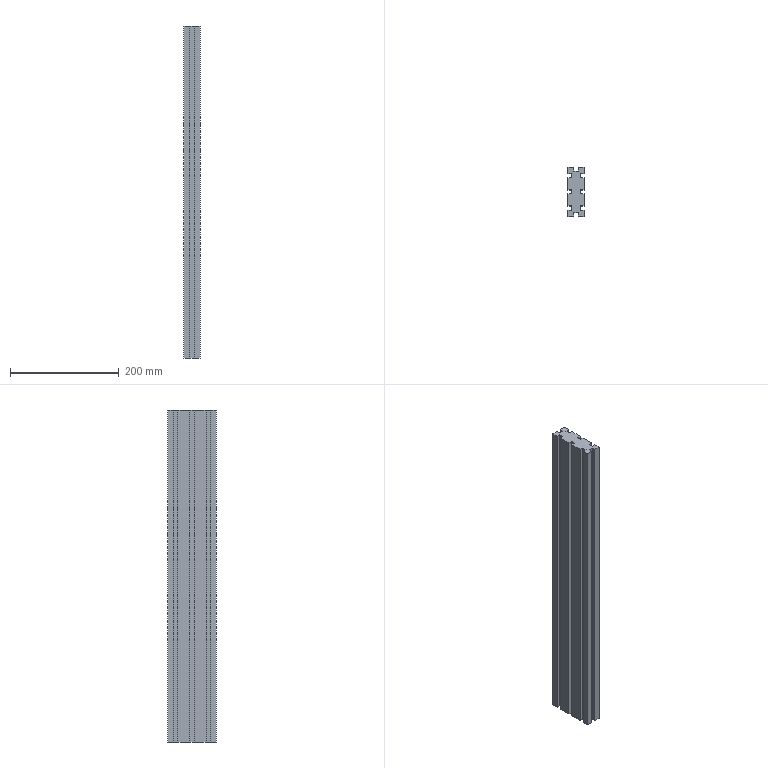Part | SolidWorks | features BaseBody 1 | 1 solid | 38 faces | box 30 x 90 x 610 mm | volume 1373720 mm3 | plane 38
STEP:
#1=CARTESIAN_POINT('',(8.,-4.,610.));
#2=VERTEX_POINT('',#1);
#3=CARTESIAN_POINT('',(15.,-4.,610.));
#4=VERTEX_POINT('',#3);
#5=CARTESIAN_POINT('',(8.,-4.,610.));
#6=DIRECTION('',(1.,0.,0.));
#7=VECTOR('',#6,1000.);
#8=LINE('',#5,#7);
#9=EDGE_CURVE('',#2,#4,#8,.T.);
#10=ORIENTED_EDGE('',*,*,#9,.T.);
#11=CARTESIAN_POINT('',(15.,-4.,0.));
#12=VERTEX_POINT('',#11);
#13=CARTESIAN_POINT('',(15.,-4.,0.));
#14=DIRECTION('',(0.,0.,1.));
#15=VECTOR('',#14,1000.);
#16=LINE('',#13,#15);
#17=EDGE_CURVE('',#12,#4,#16,.T.);
#18=ORIENTED_EDGE('',*,*,#17,.F.);
#19=CARTESIAN_POINT('',(8.,-4.,0.));
#20=VERTEX_POINT('',#19);
#21=CARTESIAN_POINT('',(8.,-4.,0.));
#22=DIRECTION('',(1.,0.,0.));
#23=VECTOR('',#22,1000.);
#24=LINE('',#21,#23);
#25=EDGE_CURVE('',#20,#12,#24,.T.);
#26=ORIENTED_EDGE('',*,*,#25,.F.);
#27=CARTESIAN_POINT('',(8.,-4.,0.));
#28=DIRECTION('',(0.,0.,1.));
#29=VECTOR('',#28,1000.);
#30=LINE('',#27,#29);
#31=EDGE_CURVE('',#20,#2,#30,.T.);
#32=ORIENTED_EDGE('',*,*,#31,.T.);
#33=EDGE_LOOP('',(#10,#18,#26,#32));
#34=FACE_OUTER_BOUND('',#33,.T.);
#35=CARTESIAN_POINT('',(8.,-4.,0.));
#36=DIRECTION('',(0.,-1.,0.));
#37=DIRECTION('',(0.,0.,-1.));
#38=AXIS2_PLACEMENT_3D('',#35,#36,#37);
#39=PLANE('',#38);
#40=ADVANCED_FACE('',(#34),#39,.F.);
#41=CARTESIAN_POINT('',(15.,4.,610.));
#42=VERTEX_POINT('',#41);
#43=CARTESIAN_POINT('',(8.,4.,610.));
#44=VERTEX_POINT('',#43);
#45=CARTESIAN_POINT('',(8.,4.,610.));
#46=DIRECTION('',(-1.,0.,0.));
#47=VECTOR('',#46,1000.);
#48=LINE('',#45,#47);
#49=EDGE_CURVE('',#42,#44,#48,.T.);
#50=ORIENTED_EDGE('',*,*,#49,.T.);
#51=CARTESIAN_POINT('',(8.,4.,0.));
#52=VERTEX_POINT('',#51);
#53=CARTESIAN_POINT('',(8.,4.,0.));
#54=DIRECTION('',(0.,0.,1.));
#55=VECTOR('',#54,1000.);
#56=LINE('',#53,#55);
#57=EDGE_CURVE('',#52,#44,#56,.T.);
#58=ORIENTED_EDGE('',*,*,#57,.F.);
#59=CARTESIAN_POINT('',(15.,4.,0.));
#60=VERTEX_POINT('',#59);
#61=CARTESIAN_POINT('',(8.,4.,0.));
#62=DIRECTION('',(-1.,0.,0.));
#63=VECTOR('',#62,1000.);
#64=LINE('',#61,#63);
#65=EDGE_CURVE('',#60,#52,#64,.T.);
#66=ORIENTED_EDGE('',*,*,#65,.F.);
#67=CARTESIAN_POINT('',(15.,4.,0.));
#68=DIRECTION('',(0.,0.,1.));
#69=VECTOR('',#68,1000.);
#70=LINE('',#67,#69);
#71=EDGE_CURVE('',#60,#42,#70,.T.);
#72=ORIENTED_EDGE('',*,*,#71,.T.);
#73=EDGE_LOOP('',(#50,#58,#66,#72));
#74=FACE_OUTER_BOUND('',#73,.T.);
#75=CARTESIAN_POINT('',(8.,4.,0.));
#76=DIRECTION('',(0.,1.,0.));
#77=DIRECTION('',(1.,0.,0.));
#78=AXIS2_PLACEMENT_3D('',#75,#76,#77);
#79=PLANE('',#78);
#80=ADVANCED_FACE('',(#74),#79,.F.);
#81=CARTESIAN_POINT('',(8.,-4.,610.));
#82=DIRECTION('',(0.,-1.,0.));
#83=VECTOR('',#82,1000.);
#84=LINE('',#81,#83);
#85=EDGE_CURVE('',#44,#2,#84,.T.);
#86=ORIENTED_EDGE('',*,*,#85,.T.);
#87=ORIENTED_EDGE('',*,*,#31,.F.);
#88=CARTESIAN_POINT('',(8.,-4.,0.));
#89=DIRECTION('',(0.,-1.,0.));
#90=VECTOR('',#89,1000.);
#91=LINE('',#88,#90);
#92=EDGE_CURVE('',#52,#20,#91,.T.);
#93=ORIENTED_EDGE('',*,*,#92,.F.);
#94=ORIENTED_EDGE('',*,*,#57,.T.);
#95=EDGE_LOOP('',(#86,#87,#93,#94));
#96=FACE_OUTER_BOUND('',#95,.T.);
#97=CARTESIAN_POINT('',(8.,-4.,0.));
#98=DIRECTION('',(-1.,0.,0.));
#99=DIRECTION('',(0.,0.,1.));
#100=AXIS2_PLACEMENT_3D('',#97,#98,#99);
#101=PLANE('',#100);
#102=ADVANCED_FACE('',(#96),#101,.F.);
#103=CARTESIAN_POINT('',(-15.,-4.,610.));
#104=VERTEX_POINT('',#103);
#105=CARTESIAN_POINT('',(-8.,-4.,610.));
#106=VERTEX_POINT('',#105);
#107=CARTESIAN_POINT('',(-15.,-4.,610.));
#108=DIRECTION('',(1.,0.,0.));
#109=VECTOR('',#108,1000.);
#110=LINE('',#107,#109);
#111=EDGE_CURVE('',#104,#106,#110,.T.);
#112=ORIENTED_EDGE('',*,*,#111,.T.);
#113=CARTESIAN_POINT('',(-8.,-4.,0.));
#114=VERTEX_POINT('',#113);
#115=CARTESIAN_POINT('',(-8.,-4.,0.));
#116=DIRECTION('',(0.,0.,1.));
#117=VECTOR('',#116,1000.);
#118=LINE('',#115,#117);
#119=EDGE_CURVE('',#114,#106,#118,.T.);
#120=ORIENTED_EDGE('',*,*,#119,.F.);
#121=CARTESIAN_POINT('',(-15.,-4.,0.));
#122=VERTEX_POINT('',#121);
#123=CARTESIAN_POINT('',(-15.,-4.,0.));
#124=DIRECTION('',(1.,0.,0.));
#125=VECTOR('',#124,1000.);
#126=LINE('',#123,#125);
#127=EDGE_CURVE('',#122,#114,#126,.T.);
#128=ORIENTED_EDGE('',*,*,#127,.F.);
#129=CARTESIAN_POINT('',(-15.,-4.,0.));
#130=DIRECTION('',(0.,0.,1.));
#131=VECTOR('',#130,1000.);
#132=LINE('',#129,#131);
#133=EDGE_CURVE('',#122,#104,#132,.T.);
#134=ORIENTED_EDGE('',*,*,#133,.T.);
#135=EDGE_LOOP('',(#112,#120,#128,#134));
#136=FACE_OUTER_BOUND('',#135,.T.);
#137=CARTESIAN_POINT('',(-15.,-4.,0.));
#138=DIRECTION('',(0.,-1.,0.));
#139=DIRECTION('',(0.,0.,-1.));
#140=AXIS2_PLACEMENT_3D('',#137,#138,#139);
#141=PLANE('',#140);
#142=ADVANCED_FACE('',(#136),#141,.F.);
#143=CARTESIAN_POINT('',(-8.,4.,610.));
#144=VERTEX_POINT('',#143);
#145=CARTESIAN_POINT('',(-8.,-4.,610.));
#146=DIRECTION('',(0.,1.,0.));
#147=VECTOR('',#146,1000.);
#148=LINE('',#145,#147);
#149=EDGE_CURVE('',#106,#144,#148,.T.);
#150=ORIENTED_EDGE('',*,*,#149,.T.);
#151=CARTESIAN_POINT('',(-8.,4.,0.));
#152=VERTEX_POINT('',#151);
#153=CARTESIAN_POINT('',(-8.,4.,0.));
#154=DIRECTION('',(0.,0.,1.));
#155=VECTOR('',#154,1000.);
#156=LINE('',#153,#155);
#157=EDGE_CURVE('',#152,#144,#156,.T.);
#158=ORIENTED_EDGE('',*,*,#157,.F.);
#159=CARTESIAN_POINT('',(-8.,-4.,0.));
#160=DIRECTION('',(0.,1.,0.));
#161=VECTOR('',#160,1000.);
#162=LINE('',#159,#161);
#163=EDGE_CURVE('',#114,#152,#162,.T.);
#164=ORIENTED_EDGE('',*,*,#163,.F.);
#165=ORIENTED_EDGE('',*,*,#119,.T.);
#166=EDGE_LOOP('',(#150,#158,#164,#165));
#167=FACE_OUTER_BOUND('',#166,.T.);
#168=CARTESIAN_POINT('',(-8.,-4.,0.));
#169=DIRECTION('',(1.,0.,0.));
#170=DIRECTION('',(0.,1.,0.));
#171=AXIS2_PLACEMENT_3D('',#168,#169,#170);
#172=PLANE('',#171);
#173=ADVANCED_FACE('',(#167),#172,.F.);
#174=CARTESIAN_POINT('',(-15.,4.,610.));
#175=VERTEX_POINT('',#174);
#176=CARTESIAN_POINT('',(-15.,4.,610.));
#177=DIRECTION('',(-1.,0.,0.));
#178=VECTOR('',#177,1000.);
#179=LINE('',#176,#178);
#180=EDGE_CURVE('',#144,#175,#179,.T.);
#181=ORIENTED_EDGE('',*,*,#180,.T.);
#182=CARTESIAN_POINT('',(-15.,4.,0.));
#183=VERTEX_POINT('',#182);
#184=CARTESIAN_POINT('',(-15.,4.,0.));
#185=DIRECTION('',(0.,0.,1.));
#186=VECTOR('',#185,1000.);
#187=LINE('',#184,#186);
#188=EDGE_CURVE('',#183,#175,#187,.T.);
#189=ORIENTED_EDGE('',*,*,#188,.F.);
#190=CARTESIAN_POINT('',(-15.,4.,0.));
#191=DIRECTION('',(-1.,0.,0.));
#192=VECTOR('',#191,1000.);
#193=LINE('',#190,#192);
#194=EDGE_CURVE('',#152,#183,#193,.T.);
#195=ORIENTED_EDGE('',*,*,#194,.F.);
#196=ORIENTED_EDGE('',*,*,#157,.T.);
#197=EDGE_LOOP('',(#181,#189,#195,#196));
#198=FACE_OUTER_BOUND('',#197,.T.);
#199=CARTESIAN_POINT('',(-15.,4.,0.));
#200=DIRECTION('',(0.,1.,0.));
#201=DIRECTION('',(1.,0.,0.));
#202=AXIS2_PLACEMENT_3D('',#199,#200,#201);
#203=PLANE('',#202);
#204=ADVANCED_FACE('',(#198),#203,.F.);
#205=CARTESIAN_POINT('',(15.,-26.,610.));
#206=VERTEX_POINT('',#205);
#207=CARTESIAN_POINT('',(8.,-26.,610.));
#208=VERTEX_POINT('',#207);
#209=CARTESIAN_POINT('',(8.,-26.,610.));
#210=DIRECTION('',(-1.,0.,0.));
#211=VECTOR('',#210,1000.);
#212=LINE('',#209,#211);
#213=EDGE_CURVE('',#206,#208,#212,.T.);
#214=ORIENTED_EDGE('',*,*,#213,.T.);
#215=CARTESIAN_POINT('',(8.,-26.,0.));
#216=VERTEX_POINT('',#215);
#217=CARTESIAN_POINT('',(8.,-26.,0.));
#218=DIRECTION('',(0.,0.,1.));
#219=VECTOR('',#218,1000.);
#220=LINE('',#217,#219);
#221=EDGE_CURVE('',#216,#208,#220,.T.);
#222=ORIENTED_EDGE('',*,*,#221,.F.);
#223=CARTESIAN_POINT('',(15.,-26.,0.));
#224=VERTEX_POINT('',#223);
#225=CARTESIAN_POINT('',(8.,-26.,0.));
#226=DIRECTION('',(-1.,0.,0.));
#227=VECTOR('',#226,1000.);
#228=LINE('',#225,#227);
#229=EDGE_CURVE('',#224,#216,#228,.T.);
#230=ORIENTED_EDGE('',*,*,#229,.F.);
#231=CARTESIAN_POINT('',(15.,-26.,0.));
#232=DIRECTION('',(0.,0.,1.));
#233=VECTOR('',#232,1000.);
#234=LINE('',#231,#233);
#235=EDGE_CURVE('',#224,#206,#234,.T.);
#236=ORIENTED_EDGE('',*,*,#235,.T.);
#237=EDGE_LOOP('',(#214,#222,#230,#236));
#238=FACE_OUTER_BOUND('',#237,.T.);
#239=CARTESIAN_POINT('',(8.,-26.,0.));
#240=DIRECTION('',(0.,1.,0.));
#241=DIRECTION('',(1.,0.,0.));
#242=AXIS2_PLACEMENT_3D('',#239,#240,#241);
#243=PLANE('',#242);
#244=ADVANCED_FACE('',(#238),#243,.F.);
#245=CARTESIAN_POINT('',(8.,-34.,610.));
#246=VERTEX_POINT('',#245);
#247=CARTESIAN_POINT('',(8.,-26.,610.));
#248=DIRECTION('',(0.,-1.,0.));
#249=VECTOR('',#248,1000.);
#250=LINE('',#247,#249);
#251=EDGE_CURVE('',#208,#246,#250,.T.);
#252=ORIENTED_EDGE('',*,*,#251,.T.);
#253=CARTESIAN_POINT('',(8.,-34.,0.));
#254=VERTEX_POINT('',#253);
#255=CARTESIAN_POINT('',(8.,-34.,0.));
#256=DIRECTION('',(0.,0.,1.));
#257=VECTOR('',#256,1000.);
#258=LINE('',#255,#257);
#259=EDGE_CURVE('',#254,#246,#258,.T.);
#260=ORIENTED_EDGE('',*,*,#259,.F.);
#261=CARTESIAN_POINT('',(8.,-26.,0.));
#262=DIRECTION('',(0.,-1.,0.));
#263=VECTOR('',#262,1000.);
#264=LINE('',#261,#263);
#265=EDGE_CURVE('',#216,#254,#264,.T.);
#266=ORIENTED_EDGE('',*,*,#265,.F.);
#267=ORIENTED_EDGE('',*,*,#221,.T.);
#268=EDGE_LOOP('',(#252,#260,#266,#267));
#269=FACE_OUTER_BOUND('',#268,.T.);
#270=CARTESIAN_POINT('',(8.,-26.,0.));
#271=DIRECTION('',(-1.,0.,0.));
#272=DIRECTION('',(0.,1.,0.));
#273=AXIS2_PLACEMENT_3D('',#270,#271,#272);
#274=PLANE('',#273);
#275=ADVANCED_FACE('',(#269),#274,.F.);
#276=CARTESIAN_POINT('',(15.,-34.,610.));
#277=VERTEX_POINT('',#276);
#278=CARTESIAN_POINT('',(8.,-34.,610.));
#279=DIRECTION('',(1.,0.,0.));
#280=VECTOR('',#279,1000.);
#281=LINE('',#278,#280);
#282=EDGE_CURVE('',#246,#277,#281,.T.);
#283=ORIENTED_EDGE('',*,*,#282,.T.);
#284=CARTESIAN_POINT('',(15.,-34.,0.));
#285=VERTEX_POINT('',#284);
#286=CARTESIAN_POINT('',(15.,-34.,0.));
#287=DIRECTION('',(0.,0.,1.));
#288=VECTOR('',#287,1000.);
#289=LINE('',#286,#288);
#290=EDGE_CURVE('',#285,#277,#289,.T.);
#291=ORIENTED_EDGE('',*,*,#290,.F.);
#292=CARTESIAN_POINT('',(8.,-34.,0.));
#293=DIRECTION('',(1.,0.,0.));
#294=VECTOR('',#293,1000.);
#295=LINE('',#292,#294);
#296=EDGE_CURVE('',#254,#285,#295,.T.);
#297=ORIENTED_EDGE('',*,*,#296,.F.);
#298=ORIENTED_EDGE('',*,*,#259,.T.);
#299=EDGE_LOOP('',(#283,#291,#297,#298));
#300=FACE_OUTER_BOUND('',#299,.T.);
#301=CARTESIAN_POINT('',(8.,-34.,0.));
#302=DIRECTION('',(0.,-1.,0.));
#303=DIRECTION('',(0.,0.,-1.));
#304=AXIS2_PLACEMENT_3D('',#301,#302,#303);
#305=PLANE('',#304);
#306=ADVANCED_FACE('',(#300),#305,.F.);
#307=CARTESIAN_POINT('',(-15.,-34.,610.));
#308=VERTEX_POINT('',#307);
#309=CARTESIAN_POINT('',(-8.,-34.,610.));
#310=VERTEX_POINT('',#309);
#311=CARTESIAN_POINT('',(-15.,-34.,610.));
#312=DIRECTION('',(1.,0.,0.));
#313=VECTOR('',#312,1000.);
#314=LINE('',#311,#313);
#315=EDGE_CURVE('',#308,#310,#314,.T.);
#316=ORIENTED_EDGE('',*,*,#315,.T.);
#317=CARTESIAN_POINT('',(-8.,-34.,0.));
#318=VERTEX_POINT('',#317);
#319=CARTESIAN_POINT('',(-8.,-34.,0.));
#320=DIRECTION('',(0.,0.,1.));
#321=VECTOR('',#320,1000.);
#322=LINE('',#319,#321);
#323=EDGE_CURVE('',#318,#310,#322,.T.);
#324=ORIENTED_EDGE('',*,*,#323,.F.);
#325=CARTESIAN_POINT('',(-15.,-34.,0.));
#326=VERTEX_POINT('',#325);
#327=CARTESIAN_POINT('',(-15.,-34.,0.));
#328=DIRECTION('',(1.,0.,0.));
#329=VECTOR('',#328,1000.);
#330=LINE('',#327,#329);
#331=EDGE_CURVE('',#326,#318,#330,.T.);
#332=ORIENTED_EDGE('',*,*,#331,.F.);
#333=CARTESIAN_POINT('',(-15.,-34.,0.));
#334=DIRECTION('',(0.,0.,1.));
#335=VECTOR('',#334,1000.);
#336=LINE('',#333,#335);
#337=EDGE_CURVE('',#326,#308,#336,.T.);
#338=ORIENTED_EDGE('',*,*,#337,.T.);
#339=EDGE_LOOP('',(#316,#324,#332,#338));
#340=FACE_OUTER_BOUND('',#339,.T.);
#341=CARTESIAN_POINT('',(-15.,-34.,0.));
#342=DIRECTION('',(0.,-1.,0.));
#343=DIRECTION('',(0.,0.,-1.));
#344=AXIS2_PLACEMENT_3D('',#341,#342,#343);
#345=PLANE('',#344);
#346=ADVANCED_FACE('',(#340),#345,.F.);
#347=CARTESIAN_POINT('',(-8.,-26.,610.));
#348=VERTEX_POINT('',#347);
#349=CARTESIAN_POINT('',(-8.,-26.,610.));
#350=DIRECTION('',(0.,1.,0.));
#351=VECTOR('',#350,1000.);
#352=LINE('',#349,#351);
#353=EDGE_CURVE('',#310,#348,#352,.T.);
#354=ORIENTED_EDGE('',*,*,#353,.T.);
#355=CARTESIAN_POINT('',(-8.,-26.,0.));
#356=VERTEX_POINT('',#355);
#357=CARTESIAN_POINT('',(-8.,-26.,0.));
#358=DIRECTION('',(0.,0.,1.));
#359=VECTOR('',#358,1000.);
#360=LINE('',#357,#359);
#361=EDGE_CURVE('',#356,#348,#360,.T.);
#362=ORIENTED_EDGE('',*,*,#361,.F.);
#363=CARTESIAN_POINT('',(-8.,-26.,0.));
#364=DIRECTION('',(0.,1.,0.));
#365=VECTOR('',#364,1000.);
#366=LINE('',#363,#365);
#367=EDGE_CURVE('',#318,#356,#366,.T.);
#368=ORIENTED_EDGE('',*,*,#367,.F.);
#369=ORIENTED_EDGE('',*,*,#323,.T.);
#370=EDGE_LOOP('',(#354,#362,#368,#369));
#371=FACE_OUTER_BOUND('',#370,.T.);
#372=CARTESIAN_POINT('',(-8.,-26.,0.));
#373=DIRECTION('',(1.,0.,0.));
#374=DIRECTION('',(0.,1.,0.));
#375=AXIS2_PLACEMENT_3D('',#372,#373,#374);
#376=PLANE('',#375);
#377=ADVANCED_FACE('',(#371),#376,.F.);
#378=CARTESIAN_POINT('',(-15.,-26.,610.));
#379=VERTEX_POINT('',#378);
#380=CARTESIAN_POINT('',(-15.,-26.,610.));
#381=DIRECTION('',(-1.,0.,0.));
#382=VECTOR('',#381,1000.);
#383=LINE('',#380,#382);
#384=EDGE_CURVE('',#348,#379,#383,.T.);
#385=ORIENTED_EDGE('',*,*,#384,.T.);
#386=CARTESIAN_POINT('',(-15.,-26.,0.));
#387=VERTEX_POINT('',#386);
#388=CARTESIAN_POINT('',(-15.,-26.,0.));
#389=DIRECTION('',(0.,0.,1.));
#390=VECTOR('',#389,1000.);
#391=LINE('',#388,#390);
#392=EDGE_CURVE('',#387,#379,#391,.T.);
#393=ORIENTED_EDGE('',*,*,#392,.F.);
#394=CARTESIAN_POINT('',(-15.,-26.,0.));
#395=DIRECTION('',(-1.,0.,0.));
#396=VECTOR('',#395,1000.);
#397=LINE('',#394,#396);
#398=EDGE_CURVE('',#356,#387,#397,.T.);
#399=ORIENTED_EDGE('',*,*,#398,.F.);
#400=ORIENTED_EDGE('',*,*,#361,.T.);
#401=EDGE_LOOP('',(#385,#393,#399,#400));
#402=FACE_OUTER_BOUND('',#401,.T.);
#403=CARTESIAN_POINT('',(-15.,-26.,0.));
#404=DIRECTION('',(0.,1.,0.));
#405=DIRECTION('',(1.,0.,0.));
#406=AXIS2_PLACEMENT_3D('',#403,#404,#405);
#407=PLANE('',#406);
#408=ADVANCED_FACE('',(#402),#407,.F.);
#409=CARTESIAN_POINT('',(15.,34.,610.));
#410=VERTEX_POINT('',#409);
#411=CARTESIAN_POINT('',(8.,34.,610.));
#412=VERTEX_POINT('',#411);
#413=CARTESIAN_POINT('',(8.,34.,610.));
#414=DIRECTION('',(-1.,0.,0.));
#415=VECTOR('',#414,1000.);
#416=LINE('',#413,#415);
#417=EDGE_CURVE('',#410,#412,#416,.T.);
#418=ORIENTED_EDGE('',*,*,#417,.T.);
#419=CARTESIAN_POINT('',(8.,34.,0.));
#420=VERTEX_POINT('',#419);
#421=CARTESIAN_POINT('',(8.,34.,0.));
#422=DIRECTION('',(0.,0.,1.));
#423=VECTOR('',#422,1000.);
#424=LINE('',#421,#423);
#425=EDGE_CURVE('',#420,#412,#424,.T.);
#426=ORIENTED_EDGE('',*,*,#425,.F.);
#427=CARTESIAN_POINT('',(15.,34.,0.));
#428=VERTEX_POINT('',#427);
#429=CARTESIAN_POINT('',(8.,34.,0.));
#430=DIRECTION('',(-1.,0.,0.));
#431=VECTOR('',#430,1000.);
#432=LINE('',#429,#431);
#433=EDGE_CURVE('',#428,#420,#432,.T.);
#434=ORIENTED_EDGE('',*,*,#433,.F.);
#435=CARTESIAN_POINT('',(15.,34.,0.));
#436=DIRECTION('',(0.,0.,1.));
#437=VECTOR('',#436,1000.);
#438=LINE('',#435,#437);
#439=EDGE_CURVE('',#428,#410,#438,.T.);
#440=ORIENTED_EDGE('',*,*,#439,.T.);
#441=EDGE_LOOP('',(#418,#426,#434,#440));
#442=FACE_OUTER_BOUND('',#441,.T.);
#443=CARTESIAN_POINT('',(8.,34.,0.));
#444=DIRECTION('',(0.,1.,0.));
#445=DIRECTION('',(1.,0.,0.));
#446=AXIS2_PLACEMENT_3D('',#443,#444,#445);
#447=PLANE('',#446);
#448=ADVANCED_FACE('',(#442),#447,.F.);
#449=CARTESIAN_POINT('',(8.,26.,610.));
#450=VERTEX_POINT('',#449);
#451=CARTESIAN_POINT('',(8.,34.,610.));
#452=DIRECTION('',(0.,-1.,0.));
#453=VECTOR('',#452,1000.);
#454=LINE('',#451,#453);
#455=EDGE_CURVE('',#412,#450,#454,.T.);
#456=ORIENTED_EDGE('',*,*,#455,.T.);
#457=CARTESIAN_POINT('',(8.,26.,0.));
#458=VERTEX_POINT('',#457);
#459=CARTESIAN_POINT('',(8.,26.,0.));
#460=DIRECTION('',(0.,0.,1.));
#461=VECTOR('',#460,1000.);
#462=LINE('',#459,#461);
#463=EDGE_CURVE('',#458,#450,#462,.T.);
#464=ORIENTED_EDGE('',*,*,#463,.F.);
#465=CARTESIAN_POINT('',(8.,34.,0.));
#466=DIRECTION('',(0.,-1.,0.));
#467=VECTOR('',#466,1000.);
#468=LINE('',#465,#467);
#469=EDGE_CURVE('',#420,#458,#468,.T.);
#470=ORIENTED_EDGE('',*,*,#469,.F.);
#471=ORIENTED_EDGE('',*,*,#425,.T.);
#472=EDGE_LOOP('',(#456,#464,#470,#471));
#473=FACE_OUTER_BOUND('',#472,.T.);
#474=CARTESIAN_POINT('',(8.,34.,0.));
#475=DIRECTION('',(-1.,0.,0.));
#476=DIRECTION('',(0.,1.,0.));
#477=AXIS2_PLACEMENT_3D('',#474,#475,#476);
#478=PLANE('',#477);
#479=ADVANCED_FACE('',(#473),#478,.F.);
#480=CARTESIAN_POINT('',(15.,26.,610.));
#481=VERTEX_POINT('',#480);
#482=CARTESIAN_POINT('',(8.,26.,610.));
#483=DIRECTION('',(1.,0.,0.));
#484=VECTOR('',#483,1000.);
#485=LINE('',#482,#484);
#486=EDGE_CURVE('',#450,#481,#485,.T.);
#487=ORIENTED_EDGE('',*,*,#486,.T.);
#488=CARTESIAN_POINT('',(15.,26.,0.));
#489=VERTEX_POINT('',#488);
#490=CARTESIAN_POINT('',(15.,26.,0.));
#491=DIRECTION('',(0.,0.,1.));
#492=VECTOR('',#491,1000.);
#493=LINE('',#490,#492);
#494=EDGE_CURVE('',#489,#481,#493,.T.);
#495=ORIENTED_EDGE('',*,*,#494,.F.);
#496=CARTESIAN_POINT('',(8.,26.,0.));
#497=DIRECTION('',(1.,0.,0.));
#498=VECTOR('',#497,1000.);
#499=LINE('',#496,#498);
#500=EDGE_CURVE('',#458,#489,#499,.T.);
#501=ORIENTED_EDGE('',*,*,#500,.F.);
#502=ORIENTED_EDGE('',*,*,#463,.T.);
#503=EDGE_LOOP('',(#487,#495,#501,#502));
#504=FACE_OUTER_BOUND('',#503,.T.);
#505=CARTESIAN_POINT('',(8.,26.,0.));
#506=DIRECTION('',(0.,-1.,0.));
#507=DIRECTION('',(0.,0.,-1.));
#508=AXIS2_PLACEMENT_3D('',#505,#506,#507);
#509=PLANE('',#508);
#510=ADVANCED_FACE('',(#504),#509,.F.);
#511=CARTESIAN_POINT('',(-15.,26.,610.));
#512=VERTEX_POINT('',#511);
#513=CARTESIAN_POINT('',(-8.,26.,610.));
#514=VERTEX_POINT('',#513);
#515=CARTESIAN_POINT('',(-15.,26.,610.));
#516=DIRECTION('',(1.,0.,0.));
#517=VECTOR('',#516,1000.);
#518=LINE('',#515,#517);
#519=EDGE_CURVE('',#512,#514,#518,.T.);
#520=ORIENTED_EDGE('',*,*,#519,.T.);
#521=CARTESIAN_POINT('',(-8.,26.,0.));
#522=VERTEX_POINT('',#521);
#523=CARTESIAN_POINT('',(-8.,26.,0.));
#524=DIRECTION('',(0.,0.,1.));
#525=VECTOR('',#524,1000.);
#526=LINE('',#523,#525);
#527=EDGE_CURVE('',#522,#514,#526,.T.);
#528=ORIENTED_EDGE('',*,*,#527,.F.);
#529=CARTESIAN_POINT('',(-15.,26.,0.));
#530=VERTEX_POINT('',#529);
#531=CARTESIAN_POINT('',(-15.,26.,0.));
#532=DIRECTION('',(1.,0.,0.));
#533=VECTOR('',#532,1000.);
#534=LINE('',#531,#533);
#535=EDGE_CURVE('',#530,#522,#534,.T.);
#536=ORIENTED_EDGE('',*,*,#535,.F.);
#537=CARTESIAN_POINT('',(-15.,26.,0.));
#538=DIRECTION('',(0.,0.,1.));
#539=VECTOR('',#538,1000.);
#540=LINE('',#537,#539);
#541=EDGE_CURVE('',#530,#512,#540,.T.);
#542=ORIENTED_EDGE('',*,*,#541,.T.);
#543=EDGE_LOOP('',(#520,#528,#536,#542));
#544=FACE_OUTER_BOUND('',#543,.T.);
#545=CARTESIAN_POINT('',(-15.,26.,0.));
#546=DIRECTION('',(0.,-1.,0.));
#547=DIRECTION('',(0.,0.,-1.));
#548=AXIS2_PLACEMENT_3D('',#545,#546,#547);
#549=PLANE('',#548);
#550=ADVANCED_FACE('',(#544),#549,.F.);
#551=CARTESIAN_POINT('',(-8.,34.,610.));
#552=VERTEX_POINT('',#551);
#553=CARTESIAN_POINT('',(-8.,34.,610.));
#554=DIRECTION('',(0.,1.,0.));
#555=VECTOR('',#554,1000.);
#556=LINE('',#553,#555);
#557=EDGE_CURVE('',#514,#552,#556,.T.);
#558=ORIENTED_EDGE('',*,*,#557,.T.);
#559=CARTESIAN_POINT('',(-8.,34.,0.));
#560=VERTEX_POINT('',#559);
#561=CARTESIAN_POINT('',(-8.,34.,0.));
#562=DIRECTION('',(0.,0.,1.));
#563=VECTOR('',#562,1000.);
#564=LINE('',#561,#563);
#565=EDGE_CURVE('',#560,#552,#564,.T.);
#566=ORIENTED_EDGE('',*,*,#565,.F.);
#567=CARTESIAN_POINT('',(-8.,34.,0.));
#568=DIRECTION('',(0.,1.,0.));
#569=VECTOR('',#568,1000.);
#570=LINE('',#567,#569);
#571=EDGE_CURVE('',#522,#560,#570,.T.);
#572=ORIENTED_EDGE('',*,*,#571,.F.);
#573=ORIENTED_EDGE('',*,*,#527,.T.);
#574=EDGE_LOOP('',(#558,#566,#572,#573));
#575=FACE_OUTER_BOUND('',#574,.T.);
#576=CARTESIAN_POINT('',(-8.,34.,0.));
#577=DIRECTION('',(1.,0.,0.));
#578=DIRECTION('',(0.,1.,0.));
#579=AXIS2_PLACEMENT_3D('',#576,#577,#578);
#580=PLANE('',#579);
#581=ADVANCED_FACE('',(#575),#580,.F.);
#582=CARTESIAN_POINT('',(-15.,34.,610.));
#583=VERTEX_POINT('',#582);
#584=CARTESIAN_POINT('',(-15.,34.,610.));
#585=DIRECTION('',(-1.,0.,0.));
#586=VECTOR('',#585,1000.);
#587=LINE('',#584,#586);
#588=EDGE_CURVE('',#552,#583,#587,.T.);
#589=ORIENTED_EDGE('',*,*,#588,.T.);
#590=CARTESIAN_POINT('',(-15.,34.,0.));
#591=VERTEX_POINT('',#590);
#592=CARTESIAN_POINT('',(-15.,34.,0.));
#593=DIRECTION('',(0.,0.,1.));
#594=VECTOR('',#593,1000.);
#595=LINE('',#592,#594);
#596=EDGE_CURVE('',#591,#583,#595,.T.);
#597=ORIENTED_EDGE('',*,*,#596,.F.);
#598=CARTESIAN_POINT('',(-15.,34.,0.));
#599=DIRECTION('',(-1.,0.,0.));
#600=VECTOR('',#599,1000.);
#601=LINE('',#598,#600);
#602=EDGE_CURVE('',#560,#591,#601,.T.);
#603=ORIENTED_EDGE('',*,*,#602,.F.);
#604=ORIENTED_EDGE('',*,*,#565,.T.);
#605=EDGE_LOOP('',(#589,#597,#603,#604));
#606=FACE_OUTER_BOUND('',#605,.T.);
#607=CARTESIAN_POINT('',(-15.,34.,0.));
#608=DIRECTION('',(0.,1.,0.));
#609=DIRECTION('',(1.,0.,0.));
#610=AXIS2_PLACEMENT_3D('',#607,#608,#609);
#611=PLANE('',#610);
#612=ADVANCED_FACE('',(#606),#611,.F.);
#613=CARTESIAN_POINT('',(4.,-45.,610.));
#614=VERTEX_POINT('',#613);
#615=CARTESIAN_POINT('',(4.,-38.,610.));
#616=VERTEX_POINT('',#615);
#617=CARTESIAN_POINT('',(4.,-38.,610.));
#618=DIRECTION('',(0.,1.,0.));
#619=VECTOR('',#618,1000.);
#620=LINE('',#617,#619);
#621=EDGE_CURVE('',#614,#616,#620,.T.);
#622=ORIENTED_EDGE('',*,*,#621,.T.);
#623=CARTESIAN_POINT('',(4.,-38.,0.));
#624=VERTEX_POINT('',#623);
#625=CARTESIAN_POINT('',(4.,-38.,0.));
#626=DIRECTION('',(0.,0.,1.));
#627=VECTOR('',#626,1000.);
#628=LINE('',#625,#627);
#629=EDGE_CURVE('',#624,#616,#628,.T.);
#630=ORIENTED_EDGE('',*,*,#629,.F.);
#631=CARTESIAN_POINT('',(4.,-45.,0.));
#632=VERTEX_POINT('',#631);
#633=CARTESIAN_POINT('',(4.,-38.,0.));
#634=DIRECTION('',(0.,1.,0.));
#635=VECTOR('',#634,1000.);
#636=LINE('',#633,#635);
#637=EDGE_CURVE('',#632,#624,#636,.T.);
#638=ORIENTED_EDGE('',*,*,#637,.F.);
#639=CARTESIAN_POINT('',(4.,-45.,0.));
#640=DIRECTION('',(0.,0.,1.));
#641=VECTOR('',#640,1000.);
#642=LINE('',#639,#641);
#643=EDGE_CURVE('',#632,#614,#642,.T.);
#644=ORIENTED_EDGE('',*,*,#643,.T.);
#645=EDGE_LOOP('',(#622,#630,#638,#644));
#646=FACE_OUTER_BOUND('',#645,.T.);
#647=CARTESIAN_POINT('',(4.,-38.,0.));
#648=DIRECTION('',(1.,0.,0.));
#649=DIRECTION('',(0.,1.,0.));
#650=AXIS2_PLACEMENT_3D('',#647,#648,#649);
#651=PLANE('',#650);
#652=ADVANCED_FACE('',(#646),#651,.F.);
#653=CARTESIAN_POINT('',(-4.,-38.,610.));
#654=VERTEX_POINT('',#653);
#655=CARTESIAN_POINT('',(-4.,-38.,610.));
#656=DIRECTION('',(-1.,0.,0.));
#657=VECTOR('',#656,1000.);
#658=LINE('',#655,#657);
#659=EDGE_CURVE('',#616,#654,#658,.T.);
#660=ORIENTED_EDGE('',*,*,#659,.T.);
#661=CARTESIAN_POINT('',(-4.,-38.,0.));
#662=VERTEX_POINT('',#661);
#663=CARTESIAN_POINT('',(-4.,-38.,0.));
#664=DIRECTION('',(0.,0.,1.));
#665=VECTOR('',#664,1000.);
#666=LINE('',#663,#665);
#667=EDGE_CURVE('',#662,#654,#666,.T.);
#668=ORIENTED_EDGE('',*,*,#667,.F.);
#669=CARTESIAN_POINT('',(-4.,-38.,0.));
#670=DIRECTION('',(-1.,0.,0.));
#671=VECTOR('',#670,1000.);
#672=LINE('',#669,#671);
#673=EDGE_CURVE('',#624,#662,#672,.T.);
#674=ORIENTED_EDGE('',*,*,#673,.F.);
#675=ORIENTED_EDGE('',*,*,#629,.T.);
#676=EDGE_LOOP('',(#660,#668,#674,#675));
#677=FACE_OUTER_BOUND('',#676,.T.);
#678=CARTESIAN_POINT('',(-4.,-38.,0.));
#679=DIRECTION('',(0.,1.,0.));
#680=DIRECTION('',(1.,0.,0.));
#681=AXIS2_PLACEMENT_3D('',#678,#679,#680);
#682=PLANE('',#681);
#683=ADVANCED_FACE('',(#677),#682,.F.);
#684=CARTESIAN_POINT('',(-4.,-45.,610.));
#685=VERTEX_POINT('',#684);
#686=CARTESIAN_POINT('',(-4.,-38.,610.));
#687=DIRECTION('',(0.,-1.,0.));
#688=VECTOR('',#687,1000.);
#689=LINE('',#686,#688);
#690=EDGE_CURVE('',#654,#685,#689,.T.);
#691=ORIENTED_EDGE('',*,*,#690,.T.);
#692=CARTESIAN_POINT('',(-4.,-45.,0.));
#693=VERTEX_POINT('',#692);
#694=CARTESIAN_POINT('',(-4.,-45.,0.));
#695=DIRECTION('',(0.,0.,1.));
#696=VECTOR('',#695,1000.);
#697=LINE('',#694,#696);
#698=EDGE_CURVE('',#693,#685,#697,.T.);
#699=ORIENTED_EDGE('',*,*,#698,.F.);
#700=CARTESIAN_POINT('',(-4.,-38.,0.));
#701=DIRECTION('',(0.,-1.,0.));
#702=VECTOR('',#701,1000.);
#703=LINE('',#700,#702);
#704=EDGE_CURVE('',#662,#693,#703,.T.);
#705=ORIENTED_EDGE('',*,*,#704,.F.);
#706=ORIENTED_EDGE('',*,*,#667,.T.);
#707=EDGE_LOOP('',(#691,#699,#705,#706));
#708=FACE_OUTER_BOUND('',#707,.T.);
#709=CARTESIAN_POINT('',(-4.,-38.,0.));
#710=DIRECTION('',(-1.,0.,0.));
#711=DIRECTION('',(0.,1.,0.));
#712=AXIS2_PLACEMENT_3D('',#709,#710,#711);
#713=PLANE('',#712);
#714=ADVANCED_FACE('',(#708),#713,.F.);
#715=CARTESIAN_POINT('',(-4.,45.,610.));
#716=VERTEX_POINT('',#715);
#717=CARTESIAN_POINT('',(-4.,38.,610.));
#718=VERTEX_POINT('',#717);
#719=CARTESIAN_POINT('',(-4.,45.,610.));
#720=DIRECTION('',(0.,-1.,0.));
#721=VECTOR('',#720,1000.);
#722=LINE('',#719,#721);
#723=EDGE_CURVE('',#716,#718,#722,.T.);
#724=ORIENTED_EDGE('',*,*,#723,.T.);
#725=CARTESIAN_POINT('',(-4.,38.,0.));
#726=VERTEX_POINT('',#725);
#727=CARTESIAN_POINT('',(-4.,38.,0.));
#728=DIRECTION('',(0.,0.,1.));
#729=VECTOR('',#728,1000.);
#730=LINE('',#727,#729);
#731=EDGE_CURVE('',#726,#718,#730,.T.);
#732=ORIENTED_EDGE('',*,*,#731,.F.);
#733=CARTESIAN_POINT('',(-4.,45.,0.));
#734=VERTEX_POINT('',#733);
#735=CARTESIAN_POINT('',(-4.,45.,0.));
#736=DIRECTION('',(0.,-1.,0.));
#737=VECTOR('',#736,1000.);
#738=LINE('',#735,#737);
#739=EDGE_CURVE('',#734,#726,#738,.T.);
#740=ORIENTED_EDGE('',*,*,#739,.F.);
#741=CARTESIAN_POINT('',(-4.,45.,0.));
#742=DIRECTION('',(0.,0.,1.));
#743=VECTOR('',#742,1000.);
#744=LINE('',#741,#743);
#745=EDGE_CURVE('',#734,#716,#744,.T.);
#746=ORIENTED_EDGE('',*,*,#745,.T.);
#747=EDGE_LOOP('',(#724,#732,#740,#746));
#748=FACE_OUTER_BOUND('',#747,.T.);
#749=CARTESIAN_POINT('',(-4.,45.,0.));
#750=DIRECTION('',(-1.,0.,0.));
#751=DIRECTION('',(0.,1.,0.));
#752=AXIS2_PLACEMENT_3D('',#749,#750,#751);
#753=PLANE('',#752);
#754=ADVANCED_FACE('',(#748),#753,.F.);
#755=CARTESIAN_POINT('',(4.,38.,610.));
#756=VERTEX_POINT('',#755);
#757=CARTESIAN_POINT('',(-4.,38.,610.));
#758=DIRECTION('',(1.,0.,0.));
#759=VECTOR('',#758,1000.);
#760=LINE('',#757,#759);
#761=EDGE_CURVE('',#718,#756,#760,.T.);
#762=ORIENTED_EDGE('',*,*,#761,.T.);
#763=CARTESIAN_POINT('',(4.,38.,0.));
#764=VERTEX_POINT('',#763);
#765=CARTESIAN_POINT('',(4.,38.,0.));
#766=DIRECTION('',(0.,0.,1.));
#767=VECTOR('',#766,1000.);
#768=LINE('',#765,#767);
#769=EDGE_CURVE('',#764,#756,#768,.T.);
#770=ORIENTED_EDGE('',*,*,#769,.F.);
#771=CARTESIAN_POINT('',(-4.,38.,0.));
#772=DIRECTION('',(1.,0.,0.));
#773=VECTOR('',#772,1000.);
#774=LINE('',#771,#773);
#775=EDGE_CURVE('',#726,#764,#774,.T.);
#776=ORIENTED_EDGE('',*,*,#775,.F.);
#777=ORIENTED_EDGE('',*,*,#731,.T.);
#778=EDGE_LOOP('',(#762,#770,#776,#777));
#779=FACE_OUTER_BOUND('',#778,.T.);
#780=CARTESIAN_POINT('',(-4.,38.,0.));
#781=DIRECTION('',(0.,-1.,0.));
#782=DIRECTION('',(0.,0.,-1.));
#783=AXIS2_PLACEMENT_3D('',#780,#781,#782);
#784=PLANE('',#783);
#785=ADVANCED_FACE('',(#779),#784,.F.);
#786=CARTESIAN_POINT('',(4.,45.,610.));
#787=VERTEX_POINT('',#786);
#788=CARTESIAN_POINT('',(4.,45.,610.));
#789=DIRECTION('',(0.,1.,0.));
#790=VECTOR('',#789,1000.);
#791=LINE('',#788,#790);
#792=EDGE_CURVE('',#756,#787,#791,.T.);
#793=ORIENTED_EDGE('',*,*,#792,.T.);
#794=CARTESIAN_POINT('',(4.,45.,0.));
#795=VERTEX_POINT('',#794);
#796=CARTESIAN_POINT('',(4.,45.,0.));
#797=DIRECTION('',(0.,0.,1.));
#798=VECTOR('',#797,1000.);
#799=LINE('',#796,#798);
#800=EDGE_CURVE('',#795,#787,#799,.T.);
#801=ORIENTED_EDGE('',*,*,#800,.F.);
#802=CARTESIAN_POINT('',(4.,45.,0.));
#803=DIRECTION('',(0.,1.,0.));
#804=VECTOR('',#803,1000.);
#805=LINE('',#802,#804);
#806=EDGE_CURVE('',#764,#795,#805,.T.);
#807=ORIENTED_EDGE('',*,*,#806,.F.);
#808=ORIENTED_EDGE('',*,*,#769,.T.);
#809=EDGE_LOOP('',(#793,#801,#807,#808));
#810=FACE_OUTER_BOUND('',#809,.T.);
#811=CARTESIAN_POINT('',(4.,45.,0.));
#812=DIRECTION('',(1.,0.,0.));
#813=DIRECTION('',(0.,1.,0.));
#814=AXIS2_PLACEMENT_3D('',#811,#812,#813);
#815=PLANE('',#814);
#816=ADVANCED_FACE('',(#810),#815,.F.);
#817=CARTESIAN_POINT('',(15.,45.,0.));
#818=DIRECTION('',(0.,1.,0.));
#819=VECTOR('',#818,1000.);
#820=LINE('',#817,#819);
#821=EDGE_CURVE('',#60,#489,#820,.T.);
#822=ORIENTED_EDGE('',*,*,#821,.F.);
#823=ORIENTED_EDGE('',*,*,#65,.T.);
#824=ORIENTED_EDGE('',*,*,#92,.T.);
#825=ORIENTED_EDGE('',*,*,#25,.T.);
#826=CARTESIAN_POINT('',(15.,45.,0.));
#827=DIRECTION('',(0.,1.,0.));
#828=VECTOR('',#827,1000.);
#829=LINE('',#826,#828);
#830=EDGE_CURVE('',#224,#12,#829,.T.);
#831=ORIENTED_EDGE('',*,*,#830,.F.);
#832=ORIENTED_EDGE('',*,*,#229,.T.);
#833=ORIENTED_EDGE('',*,*,#265,.T.);
#834=ORIENTED_EDGE('',*,*,#296,.T.);
#835=CARTESIAN_POINT('',(15.,-45.,0.));
#836=VERTEX_POINT('',#835);
#837=CARTESIAN_POINT('',(15.,45.,0.));
#838=DIRECTION('',(0.,1.,0.));
#839=VECTOR('',#838,1000.);
#840=LINE('',#837,#839);
#841=EDGE_CURVE('',#836,#285,#840,.T.);
#842=ORIENTED_EDGE('',*,*,#841,.F.);
#843=CARTESIAN_POINT('',(-15.,-45.,0.));
#844=DIRECTION('',(1.,0.,0.));
#845=VECTOR('',#844,1000.);
#846=LINE('',#843,#845);
#847=EDGE_CURVE('',#632,#836,#846,.T.);
#848=ORIENTED_EDGE('',*,*,#847,.F.);
#849=ORIENTED_EDGE('',*,*,#637,.T.);
#850=ORIENTED_EDGE('',*,*,#673,.T.);
#851=ORIENTED_EDGE('',*,*,#704,.T.);
#852=CARTESIAN_POINT('',(-15.,-45.,0.));
#853=VERTEX_POINT('',#852);
#854=CARTESIAN_POINT('',(-15.,-45.,0.));
#855=DIRECTION('',(1.,0.,0.));
#856=VECTOR('',#855,1000.);
#857=LINE('',#854,#856);
#858=EDGE_CURVE('',#853,#693,#857,.T.);
#859=ORIENTED_EDGE('',*,*,#858,.F.);
#860=CARTESIAN_POINT('',(-15.,45.,0.));
#861=DIRECTION('',(0.,-1.,0.));
#862=VECTOR('',#861,1000.);
#863=LINE('',#860,#862);
#864=EDGE_CURVE('',#326,#853,#863,.T.);
#865=ORIENTED_EDGE('',*,*,#864,.F.);
#866=ORIENTED_EDGE('',*,*,#331,.T.);
#867=ORIENTED_EDGE('',*,*,#367,.T.);
#868=ORIENTED_EDGE('',*,*,#398,.T.);
#869=CARTESIAN_POINT('',(-15.,45.,0.));
#870=DIRECTION('',(0.,-1.,0.));
#871=VECTOR('',#870,1000.);
#872=LINE('',#869,#871);
#873=EDGE_CURVE('',#122,#387,#872,.T.);
#874=ORIENTED_EDGE('',*,*,#873,.F.);
#875=ORIENTED_EDGE('',*,*,#127,.T.);
#876=ORIENTED_EDGE('',*,*,#163,.T.);
#877=ORIENTED_EDGE('',*,*,#194,.T.);
#878=CARTESIAN_POINT('',(-15.,45.,0.));
#879=DIRECTION('',(0.,-1.,0.));
#880=VECTOR('',#879,1000.);
#881=LINE('',#878,#880);
#882=EDGE_CURVE('',#530,#183,#881,.T.);
#883=ORIENTED_EDGE('',*,*,#882,.F.);
#884=ORIENTED_EDGE('',*,*,#535,.T.);
#885=ORIENTED_EDGE('',*,*,#571,.T.);
#886=ORIENTED_EDGE('',*,*,#602,.T.);
#887=CARTESIAN_POINT('',(-15.,45.,0.));
#888=VERTEX_POINT('',#887);
#889=CARTESIAN_POINT('',(-15.,45.,0.));
#890=DIRECTION('',(0.,-1.,0.));
#891=VECTOR('',#890,1000.);
#892=LINE('',#889,#891);
#893=EDGE_CURVE('',#888,#591,#892,.T.);
#894=ORIENTED_EDGE('',*,*,#893,.F.);
#895=CARTESIAN_POINT('',(-15.,45.,0.));
#896=DIRECTION('',(-1.,0.,0.));
#897=VECTOR('',#896,1000.);
#898=LINE('',#895,#897);
#899=EDGE_CURVE('',#734,#888,#898,.T.);
#900=ORIENTED_EDGE('',*,*,#899,.F.);
#901=ORIENTED_EDGE('',*,*,#739,.T.);
#902=ORIENTED_EDGE('',*,*,#775,.T.);
#903=ORIENTED_EDGE('',*,*,#806,.T.);
#904=CARTESIAN_POINT('',(15.,45.,0.));
#905=VERTEX_POINT('',#904);
#906=CARTESIAN_POINT('',(-15.,45.,0.));
#907=DIRECTION('',(-1.,0.,0.));
#908=VECTOR('',#907,1000.);
#909=LINE('',#906,#908);
#910=EDGE_CURVE('',#905,#795,#909,.T.);
#911=ORIENTED_EDGE('',*,*,#910,.F.);
#912=CARTESIAN_POINT('',(15.,45.,0.));
#913=DIRECTION('',(0.,1.,0.));
#914=VECTOR('',#913,1000.);
#915=LINE('',#912,#914);
#916=EDGE_CURVE('',#428,#905,#915,.T.);
#917=ORIENTED_EDGE('',*,*,#916,.F.);
#918=ORIENTED_EDGE('',*,*,#433,.T.);
#919=ORIENTED_EDGE('',*,*,#469,.T.);
#920=ORIENTED_EDGE('',*,*,#500,.T.);
#921=EDGE_LOOP('',(#822,#823,#824,#825,#831,#832,#833,#834,#842,#848,#849,#850,#851,#859,#865,#866,#867,#868,#874,#875,#876,#877,#883,#884,#885,#886,#894,#900,#901,#902,#903,#911,#917,#918,#919,#920));
#922=FACE_OUTER_BOUND('',#921,.T.);
#923=CARTESIAN_POINT('',(0.,0.,0.));
#924=DIRECTION('',(0.,0.,1.));
#925=DIRECTION('',(1.,0.,0.));
#926=AXIS2_PLACEMENT_3D('',#923,#924,#925);
#927=PLANE('',#926);
#928=ADVANCED_FACE('',(#922),#927,.F.);
#929=ORIENTED_EDGE('',*,*,#49,.F.);
#930=CARTESIAN_POINT('',(15.,45.,610.));
#931=DIRECTION('',(0.,1.,0.));
#932=VECTOR('',#931,1000.);
#933=LINE('',#930,#932);
#934=EDGE_CURVE('',#42,#481,#933,.T.);
#935=ORIENTED_EDGE('',*,*,#934,.T.);
#936=ORIENTED_EDGE('',*,*,#486,.F.);
#937=ORIENTED_EDGE('',*,*,#455,.F.);
#938=ORIENTED_EDGE('',*,*,#417,.F.);
#939=CARTESIAN_POINT('',(15.,45.,610.));
#940=VERTEX_POINT('',#939);
#941=CARTESIAN_POINT('',(15.,45.,610.));
#942=DIRECTION('',(0.,1.,0.));
#943=VECTOR('',#942,1000.);
#944=LINE('',#941,#943);
#945=EDGE_CURVE('',#410,#940,#944,.T.);
#946=ORIENTED_EDGE('',*,*,#945,.T.);
#947=CARTESIAN_POINT('',(-15.,45.,610.));
#948=DIRECTION('',(-1.,0.,0.));
#949=VECTOR('',#948,1000.);
#950=LINE('',#947,#949);
#951=EDGE_CURVE('',#940,#787,#950,.T.);
#952=ORIENTED_EDGE('',*,*,#951,.T.);
#953=ORIENTED_EDGE('',*,*,#792,.F.);
#954=ORIENTED_EDGE('',*,*,#761,.F.);
#955=ORIENTED_EDGE('',*,*,#723,.F.);
#956=CARTESIAN_POINT('',(-15.,45.,610.));
#957=VERTEX_POINT('',#956);
#958=CARTESIAN_POINT('',(-15.,45.,610.));
#959=DIRECTION('',(-1.,0.,0.));
#960=VECTOR('',#959,1000.);
#961=LINE('',#958,#960);
#962=EDGE_CURVE('',#716,#957,#961,.T.);
#963=ORIENTED_EDGE('',*,*,#962,.T.);
#964=CARTESIAN_POINT('',(-15.,45.,610.));
#965=DIRECTION('',(0.,-1.,0.));
#966=VECTOR('',#965,1000.);
#967=LINE('',#964,#966);
#968=EDGE_CURVE('',#957,#583,#967,.T.);
#969=ORIENTED_EDGE('',*,*,#968,.T.);
#970=ORIENTED_EDGE('',*,*,#588,.F.);
#971=ORIENTED_EDGE('',*,*,#557,.F.);
#972=ORIENTED_EDGE('',*,*,#519,.F.);
#973=CARTESIAN_POINT('',(-15.,45.,610.));
#974=DIRECTION('',(0.,-1.,0.));
#975=VECTOR('',#974,1000.);
#976=LINE('',#973,#975);
#977=EDGE_CURVE('',#512,#175,#976,.T.);
#978=ORIENTED_EDGE('',*,*,#977,.T.);
#979=ORIENTED_EDGE('',*,*,#180,.F.);
#980=ORIENTED_EDGE('',*,*,#149,.F.);
#981=ORIENTED_EDGE('',*,*,#111,.F.);
#982=CARTESIAN_POINT('',(-15.,45.,610.));
#983=DIRECTION('',(0.,-1.,0.));
#984=VECTOR('',#983,1000.);
#985=LINE('',#982,#984);
#986=EDGE_CURVE('',#104,#379,#985,.T.);
#987=ORIENTED_EDGE('',*,*,#986,.T.);
#988=ORIENTED_EDGE('',*,*,#384,.F.);
#989=ORIENTED_EDGE('',*,*,#353,.F.);
#990=ORIENTED_EDGE('',*,*,#315,.F.);
#991=CARTESIAN_POINT('',(-15.,-45.,610.));
#992=VERTEX_POINT('',#991);
#993=CARTESIAN_POINT('',(-15.,45.,610.));
#994=DIRECTION('',(0.,-1.,0.));
#995=VECTOR('',#994,1000.);
#996=LINE('',#993,#995);
#997=EDGE_CURVE('',#308,#992,#996,.T.);
#998=ORIENTED_EDGE('',*,*,#997,.T.);
#999=CARTESIAN_POINT('',(-15.,-45.,610.));
#1000=DIRECTION('',(1.,0.,0.));
#1001=VECTOR('',#1000,1000.);
#1002=LINE('',#999,#1001);
#1003=EDGE_CURVE('',#992,#685,#1002,.T.);
#1004=ORIENTED_EDGE('',*,*,#1003,.T.);
#1005=ORIENTED_EDGE('',*,*,#690,.F.);
#1006=ORIENTED_EDGE('',*,*,#659,.F.);
#1007=ORIENTED_EDGE('',*,*,#621,.F.);
#1008=CARTESIAN_POINT('',(15.,-45.,610.));
#1009=VERTEX_POINT('',#1008);
#1010=CARTESIAN_POINT('',(-15.,-45.,610.));
#1011=DIRECTION('',(1.,0.,0.));
#1012=VECTOR('',#1011,1000.);
#1013=LINE('',#1010,#1012);
#1014=EDGE_CURVE('',#614,#1009,#1013,.T.);
#1015=ORIENTED_EDGE('',*,*,#1014,.T.);
#1016=CARTESIAN_POINT('',(15.,45.,610.));
#1017=DIRECTION('',(0.,1.,0.));
#1018=VECTOR('',#1017,1000.);
#1019=LINE('',#1016,#1018);
#1020=EDGE_CURVE('',#1009,#277,#1019,.T.);
#1021=ORIENTED_EDGE('',*,*,#1020,.T.);
#1022=ORIENTED_EDGE('',*,*,#282,.F.);
#1023=ORIENTED_EDGE('',*,*,#251,.F.);
#1024=ORIENTED_EDGE('',*,*,#213,.F.);
#1025=CARTESIAN_POINT('',(15.,45.,610.));
#1026=DIRECTION('',(0.,1.,0.));
#1027=VECTOR('',#1026,1000.);
#1028=LINE('',#1025,#1027);
#1029=EDGE_CURVE('',#206,#4,#1028,.T.);
#1030=ORIENTED_EDGE('',*,*,#1029,.T.);
#1031=ORIENTED_EDGE('',*,*,#9,.F.);
#1032=ORIENTED_EDGE('',*,*,#85,.F.);
#1033=EDGE_LOOP('',(#929,#935,#936,#937,#938,#946,#952,#953,#954,#955,#963,#969,#970,#971,#972,#978,#979,#980,#981,#987,#988,#989,#990,#998,#1004,#1005,#1006,#1007,#1015,#1021,#1022,#1023,#1024,#1030,#1031,#1032));
#1034=FACE_OUTER_BOUND('',#1033,.T.);
#1035=CARTESIAN_POINT('',(0.,0.,610.));
#1036=DIRECTION('',(0.,0.,1.));
#1037=DIRECTION('',(1.,0.,0.));
#1038=AXIS2_PLACEMENT_3D('',#1035,#1036,#1037);
#1039=PLANE('',#1038);
#1040=ADVANCED_FACE('',(#1034),#1039,.T.);
#1041=ORIENTED_EDGE('',*,*,#1014,.F.);
#1042=ORIENTED_EDGE('',*,*,#643,.F.);
#1043=ORIENTED_EDGE('',*,*,#847,.T.);
#1044=CARTESIAN_POINT('',(15.,-45.,610.));
#1045=DIRECTION('',(0.,0.,-1.));
#1046=VECTOR('',#1045,1000.);
#1047=LINE('',#1044,#1046);
#1048=EDGE_CURVE('',#1009,#836,#1047,.T.);
#1049=ORIENTED_EDGE('',*,*,#1048,.F.);
#1050=EDGE_LOOP('',(#1041,#1042,#1043,#1049));
#1051=FACE_OUTER_BOUND('',#1050,.T.);
#1052=CARTESIAN_POINT('',(-15.,-45.,610.));
#1053=DIRECTION('',(0.,1.,0.));
#1054=DIRECTION('',(1.,0.,0.));
#1055=AXIS2_PLACEMENT_3D('',#1052,#1053,#1054);
#1056=PLANE('',#1055);
#1057=ADVANCED_FACE('',(#1051),#1056,.F.);
#1058=ORIENTED_EDGE('',*,*,#997,.F.);
#1059=ORIENTED_EDGE('',*,*,#337,.F.);
#1060=ORIENTED_EDGE('',*,*,#864,.T.);
#1061=CARTESIAN_POINT('',(-15.,-45.,610.));
#1062=DIRECTION('',(0.,0.,-1.));
#1063=VECTOR('',#1062,1000.);
#1064=LINE('',#1061,#1063);
#1065=EDGE_CURVE('',#992,#853,#1064,.T.);
#1066=ORIENTED_EDGE('',*,*,#1065,.F.);
#1067=EDGE_LOOP('',(#1058,#1059,#1060,#1066));
#1068=FACE_OUTER_BOUND('',#1067,.T.);
#1069=CARTESIAN_POINT('',(-15.,45.,610.));
#1070=DIRECTION('',(1.,0.,0.));
#1071=DIRECTION('',(0.,1.,0.));
#1072=AXIS2_PLACEMENT_3D('',#1069,#1070,#1071);
#1073=PLANE('',#1072);
#1074=ADVANCED_FACE('',(#1068),#1073,.F.);
#1075=ORIENTED_EDGE('',*,*,#962,.F.);
#1076=ORIENTED_EDGE('',*,*,#745,.F.);
#1077=ORIENTED_EDGE('',*,*,#899,.T.);
#1078=CARTESIAN_POINT('',(-15.,45.,610.));
#1079=DIRECTION('',(0.,0.,-1.));
#1080=VECTOR('',#1079,1000.);
#1081=LINE('',#1078,#1080);
#1082=EDGE_CURVE('',#957,#888,#1081,.T.);
#1083=ORIENTED_EDGE('',*,*,#1082,.F.);
#1084=EDGE_LOOP('',(#1075,#1076,#1077,#1083));
#1085=FACE_OUTER_BOUND('',#1084,.T.);
#1086=CARTESIAN_POINT('',(-15.,45.,610.));
#1087=DIRECTION('',(0.,-1.,0.));
#1088=DIRECTION('',(0.,0.,-1.));
#1089=AXIS2_PLACEMENT_3D('',#1086,#1087,#1088);
#1090=PLANE('',#1089);
#1091=ADVANCED_FACE('',(#1085),#1090,.F.);
#1092=ORIENTED_EDGE('',*,*,#945,.F.);
#1093=ORIENTED_EDGE('',*,*,#439,.F.);
#1094=ORIENTED_EDGE('',*,*,#916,.T.);
#1095=CARTESIAN_POINT('',(15.,45.,610.));
#1096=DIRECTION('',(0.,0.,-1.));
#1097=VECTOR('',#1096,1000.);
#1098=LINE('',#1095,#1097);
#1099=EDGE_CURVE('',#940,#905,#1098,.T.);
#1100=ORIENTED_EDGE('',*,*,#1099,.F.);
#1101=EDGE_LOOP('',(#1092,#1093,#1094,#1100));
#1102=FACE_OUTER_BOUND('',#1101,.T.);
#1103=CARTESIAN_POINT('',(15.,45.,610.));
#1104=DIRECTION('',(-1.,0.,0.));
#1105=DIRECTION('',(0.,1.,0.));
#1106=AXIS2_PLACEMENT_3D('',#1103,#1104,#1105);
#1107=PLANE('',#1106);
#1108=ADVANCED_FACE('',(#1102),#1107,.F.);
#1109=ORIENTED_EDGE('',*,*,#910,.T.);
#1110=ORIENTED_EDGE('',*,*,#800,.T.);
#1111=ORIENTED_EDGE('',*,*,#951,.F.);
#1112=ORIENTED_EDGE('',*,*,#1099,.T.);
#1113=EDGE_LOOP('',(#1109,#1110,#1111,#1112));
#1114=FACE_OUTER_BOUND('',#1113,.T.);
#1115=CARTESIAN_POINT('',(-15.,45.,610.));
#1116=DIRECTION('',(0.,-1.,0.));
#1117=DIRECTION('',(0.,0.,-1.));
#1118=AXIS2_PLACEMENT_3D('',#1115,#1116,#1117);
#1119=PLANE('',#1118);
#1120=ADVANCED_FACE('',(#1114),#1119,.F.);
#1121=ORIENTED_EDGE('',*,*,#858,.T.);
#1122=ORIENTED_EDGE('',*,*,#698,.T.);
#1123=ORIENTED_EDGE('',*,*,#1003,.F.);
#1124=ORIENTED_EDGE('',*,*,#1065,.T.);
#1125=EDGE_LOOP('',(#1121,#1122,#1123,#1124));
#1126=FACE_OUTER_BOUND('',#1125,.T.);
#1127=CARTESIAN_POINT('',(-15.,-45.,610.));
#1128=DIRECTION('',(0.,1.,0.));
#1129=DIRECTION('',(1.,0.,0.));
#1130=AXIS2_PLACEMENT_3D('',#1127,#1128,#1129);
#1131=PLANE('',#1130);
#1132=ADVANCED_FACE('',(#1126),#1131,.F.);
#1133=ORIENTED_EDGE('',*,*,#893,.T.);
#1134=ORIENTED_EDGE('',*,*,#596,.T.);
#1135=ORIENTED_EDGE('',*,*,#968,.F.);
#1136=ORIENTED_EDGE('',*,*,#1082,.T.);
#1137=EDGE_LOOP('',(#1133,#1134,#1135,#1136));
#1138=FACE_OUTER_BOUND('',#1137,.T.);
#1139=CARTESIAN_POINT('',(-15.,45.,610.));
#1140=DIRECTION('',(1.,0.,0.));
#1141=DIRECTION('',(0.,1.,0.));
#1142=AXIS2_PLACEMENT_3D('',#1139,#1140,#1141);
#1143=PLANE('',#1142);
#1144=ADVANCED_FACE('',(#1138),#1143,.F.);
#1145=ORIENTED_EDGE('',*,*,#830,.T.);
#1146=ORIENTED_EDGE('',*,*,#17,.T.);
#1147=ORIENTED_EDGE('',*,*,#1029,.F.);
#1148=ORIENTED_EDGE('',*,*,#235,.F.);
#1149=EDGE_LOOP('',(#1145,#1146,#1147,#1148));
#1150=FACE_OUTER_BOUND('',#1149,.T.);
#1151=CARTESIAN_POINT('',(15.,45.,610.));
#1152=DIRECTION('',(-1.,0.,0.));
#1153=DIRECTION('',(0.,1.,0.));
#1154=AXIS2_PLACEMENT_3D('',#1151,#1152,#1153);
#1155=PLANE('',#1154);
#1156=ADVANCED_FACE('',(#1150),#1155,.F.);
#1157=ORIENTED_EDGE('',*,*,#986,.F.);
#1158=ORIENTED_EDGE('',*,*,#133,.F.);
#1159=ORIENTED_EDGE('',*,*,#873,.T.);
#1160=ORIENTED_EDGE('',*,*,#392,.T.);
#1161=EDGE_LOOP('',(#1157,#1158,#1159,#1160));
#1162=FACE_OUTER_BOUND('',#1161,.T.);
#1163=CARTESIAN_POINT('',(-15.,45.,610.));
#1164=DIRECTION('',(1.,0.,0.));
#1165=DIRECTION('',(0.,1.,0.));
#1166=AXIS2_PLACEMENT_3D('',#1163,#1164,#1165);
#1167=PLANE('',#1166);
#1168=ADVANCED_FACE('',(#1162),#1167,.F.);
#1169=ORIENTED_EDGE('',*,*,#841,.T.);
#1170=ORIENTED_EDGE('',*,*,#290,.T.);
#1171=ORIENTED_EDGE('',*,*,#1020,.F.);
#1172=ORIENTED_EDGE('',*,*,#1048,.T.);
#1173=EDGE_LOOP('',(#1169,#1170,#1171,#1172));
#1174=FACE_OUTER_BOUND('',#1173,.T.);
#1175=CARTESIAN_POINT('',(15.,45.,610.));
#1176=DIRECTION('',(-1.,0.,0.));
#1177=DIRECTION('',(0.,1.,0.));
#1178=AXIS2_PLACEMENT_3D('',#1175,#1176,#1177);
#1179=PLANE('',#1178);
#1180=ADVANCED_FACE('',(#1174),#1179,.F.);
#1181=ORIENTED_EDGE('',*,*,#882,.T.);
#1182=ORIENTED_EDGE('',*,*,#188,.T.);
#1183=ORIENTED_EDGE('',*,*,#977,.F.);
#1184=ORIENTED_EDGE('',*,*,#541,.F.);
#1185=EDGE_LOOP('',(#1181,#1182,#1183,#1184));
#1186=FACE_OUTER_BOUND('',#1185,.T.);
#1187=CARTESIAN_POINT('',(-15.,45.,610.));
#1188=DIRECTION('',(1.,0.,0.));
#1189=DIRECTION('',(0.,1.,0.));
#1190=AXIS2_PLACEMENT_3D('',#1187,#1188,#1189);
#1191=PLANE('',#1190);
#1192=ADVANCED_FACE('',(#1186),#1191,.F.);
#1193=ORIENTED_EDGE('',*,*,#934,.F.);
#1194=ORIENTED_EDGE('',*,*,#71,.F.);
#1195=ORIENTED_EDGE('',*,*,#821,.T.);
#1196=ORIENTED_EDGE('',*,*,#494,.T.);
#1197=EDGE_LOOP('',(#1193,#1194,#1195,#1196));
#1198=FACE_OUTER_BOUND('',#1197,.T.);
#1199=CARTESIAN_POINT('',(15.,45.,610.));
#1200=DIRECTION('',(-1.,0.,0.));
#1201=DIRECTION('',(0.,1.,0.));
#1202=AXIS2_PLACEMENT_3D('',#1199,#1200,#1201);
#1203=PLANE('',#1202);
#1204=ADVANCED_FACE('',(#1198),#1203,.F.);
#1205=CLOSED_SHELL('',(#40,#80,#102,#142,#173,#204,#244,#275,#306,#346,#377,#408,#448,#479,#510,#550,#581,#612,#652,#683,#714,#754,#785,#816,#928,#1040,#1057,#1074,#1091,#1108,#1120,#1132,#1144,#1156,#1168,#1180,#1192,#1204));
#1206=MANIFOLD_SOLID_BREP('',#1205);
#1207=CARTESIAN_POINT('',(0.,0.,0.));
#1208=DIRECTION('',(0.,0.,1.));
#1209=DIRECTION('',(1.,0.,0.));
#1210=AXIS2_PLACEMENT_3D('',#1207,#1208,#1209);
#1211=(LENGTH_UNIT()NAMED_UNIT(*)SI_UNIT(.MILLI.,.METRE.));
#1212=UNCERTAINTY_MEASURE_WITH_UNIT(LENGTH_MEASURE(0.00001),#1211,'','');
#1213=(NAMED_UNIT(*)PLANE_ANGLE_UNIT()SI_UNIT($,.RADIAN.));
#1214=(NAMED_UNIT(*)SI_UNIT($,.STERADIAN.)SOLID_ANGLE_UNIT());
#1215=(GEOMETRIC_REPRESENTATION_CONTEXT(3)GLOBAL_UNCERTAINTY_ASSIGNED_CONTEXT((#1212))GLOBAL_UNIT_ASSIGNED_CONTEXT((#1211,#1213,#1214))REPRESENTATION_CONTEXT('',''));
#1216=ADVANCED_BREP_SHAPE_REPRESENTATION('',(#1206,#1210),#1215);